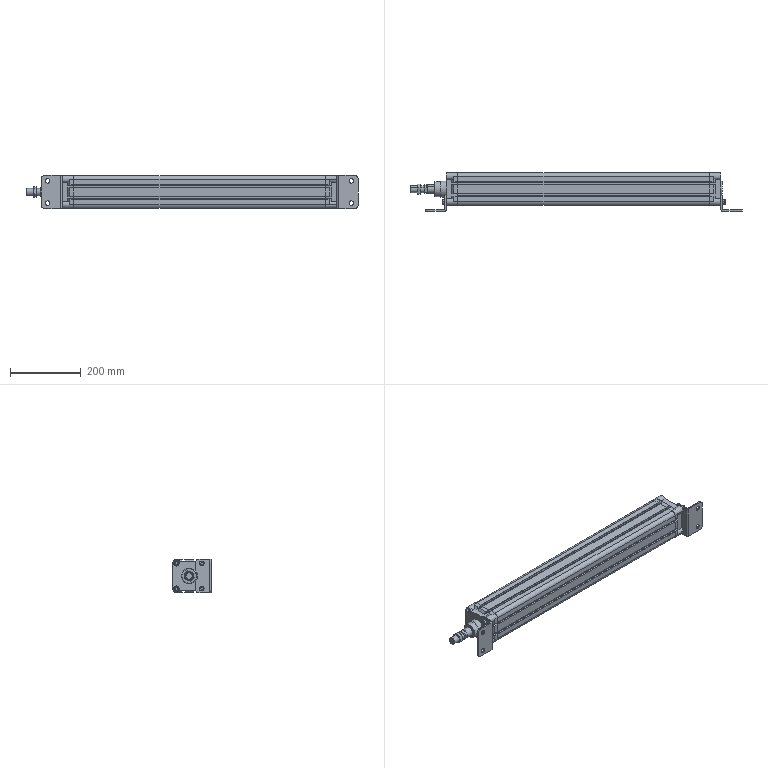Part | NX | features BREP 5 | 9 solids | 569 faces | box 940.75 x 109.5 x 95 mm | volume 3539235 mm3 | plane 253 | cylinder 248 | cone 58 | torus 10 | commonest cylinder face diameters 1 x102 8.376 x16 15.9 x16 22 x16 10 x10 20 x10